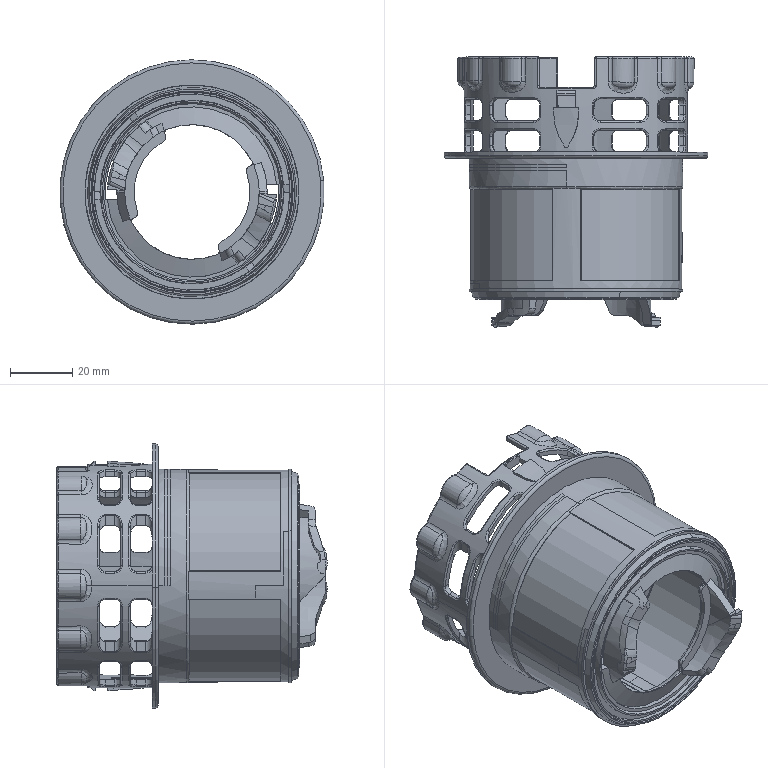Part | STEP file | ZXW722-L-24 | 1 solid | 697 faces | box 84.8 x 86.614 x 84.8 mm | volume 30515 mm3 | cylinder 208 | plane 183 | spline 180 | torus 70 | cone 42 | sphere 8 | other 6 | commonest cylinder face diameters 4 x64 1 x56 10 x10 2 x8 62 x8 62.447 x8